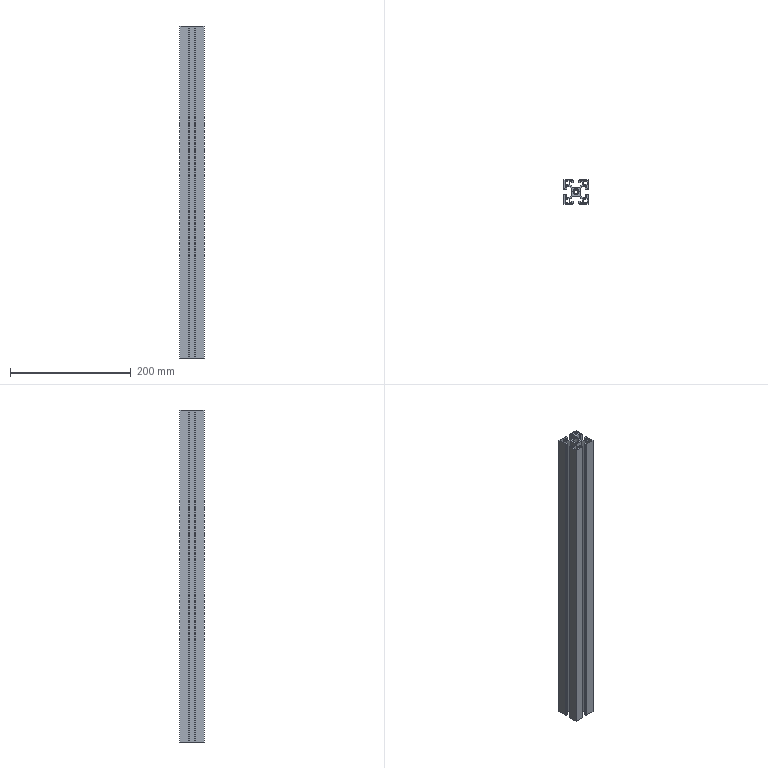Part | SolidWorks | features HoleWzd 3, Fillet 2, ICE 2, CirPattern 1, Extrusion 1, LPattern 1 | 1 solid | 108 faces | box 40 x 40 x 551 mm | volume 331194 mm3 | plane 94 | cylinder 10 | cone 4 | commonest cylinder face diameters 1 x4 6.5 x2 6.8 x2 10.2 x2